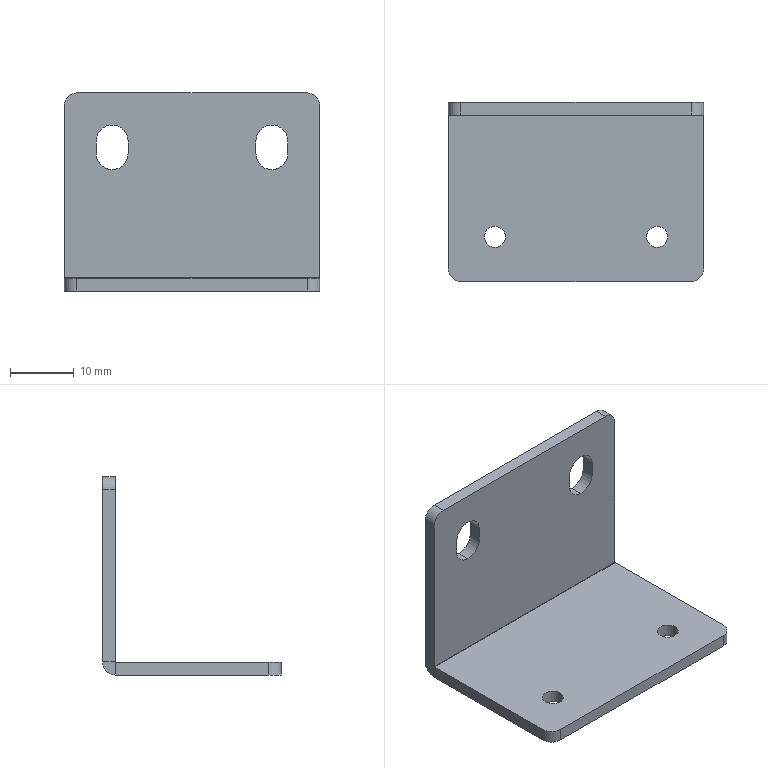Part | STEP file | Limit switch mounting plate | 1 solid | 32 faces | box 40 x 28 x 31 mm | volume 4364 mm3 | cylinder 16 | plane 16 | commonest cylinder face diameters 5 x6 3.3 x4 4 x4 0.1 x1 4.1 x1